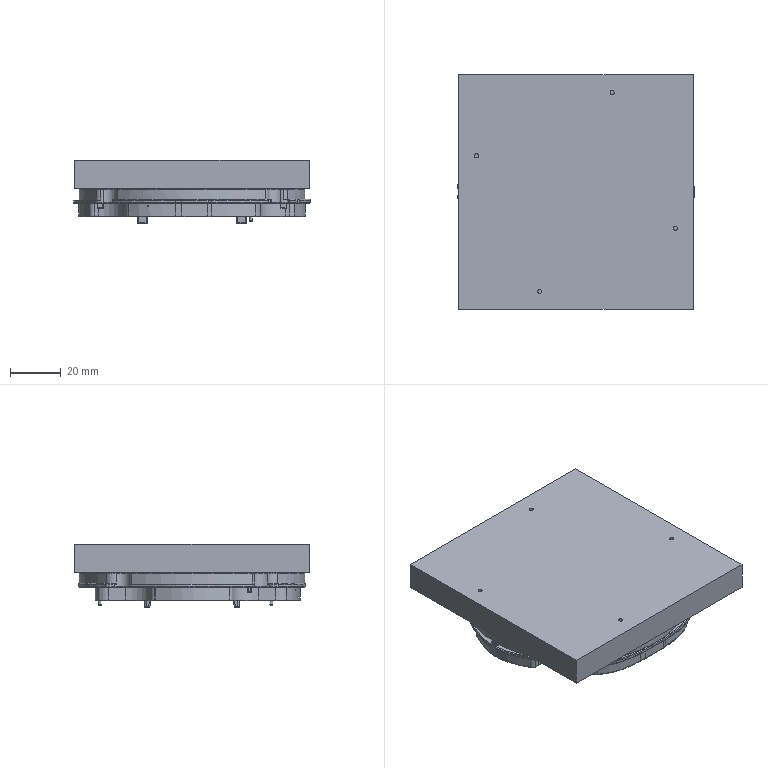NC program | NX | posted with a generic post | part box 92.935 x 92.1 x 24.829 mm
Lines 20379 to 21644 of 39008:
(PLANAR_MILL_5 , TOOL : D2-6-D4-50-3T-ROUGH)
N40738 T19 M6
N40740 G54
N40742 G17 G0 G90 X-18.001 Y31.511 S4500 M3
N40744 G43 Z20. H19
N40746 Z-3.15
N40748 G94 G1 Z-6.15 F1200.
N40750 X-16.001
N40752 X22.11
N40754 G2 X21.293 Y32.011 R2.814
N40756 G1 X-16.001
N40758 X-18.001
N40760 Z-3.15
N40762 G0 Z20.
N40764 Y27.511
N40766 Z-3.15
N40768 G1 Z-6.15
N40770 X-16.001
N40772 X24.224
N40774 Y28.011
N40776 X-16.001
N40778 X-18.001
N40780 Z-3.15
N40782 G0 Z20.
N40784 X-10.2 Y20.011
N40786 Z-3.15
N40788 G1 Z-6.15
N40790 X-12.2
N40792 X-22.92
N40794 G2 X-23.664 Y19.499 R3.
N40796 G1 X-12.2
N40798 X-10.2
N40800 Z-3.15
N40802 G0 Z20.
N40804 Y12.011
N40806 Z-3.15
N40808 G1 Z-6.15
N40810 X-12.2
N40812 X-38.698
N40814 G3 X-38.895 Y11.588 R81.553
N40816 G1 X-38.93 Y11.511
N40818 X-12.2
N40820 X-10.2
N40822 Z-3.15
N40824 G0 Z20.
N40826 Y8.011
N40828 Z-3.15
N40830 G1 Z-6.15
N40832 X-12.2
N40834 X-40.408
N40836 X-40.446 Y7.907
N40838 X-40.491 Y7.785
N40840 X-40.536 Y7.662
N40842 X-40.59 Y7.511
N40844 X-12.2
N40846 X-10.2
N40848 Z-3.15
N40850 G0 Z20.
N40852 Y4.011
N40854 Z-3.15
N40856 G1 Z-6.15
N40858 X-12.2
N40860 X-41.583
N40862 X-41.598 Y3.939
N40864 X-41.621 Y3.819
N40866 X-41.644 Y3.7
N40868 X-41.666 Y3.58
N40870 X-41.679 Y3.511
N40872 X-12.2
N40874 X-10.2
N40876 Z-3.15
N40878 G0 Z20.
N40880 Y0.011
N40882 Z-3.15
N40884 G1 Z-6.15
N40886 X-12.2
N40888 X-42.001 Y0.01
N40890 X-42. Y-0.108
N40892 X-41.999 Y-0.227
N40894 X-41.997 Y-0.345
N40896 X-41.994 Y-0.489
N40898 X-12.2
N40900 X-10.2
N40902 Z-3.15
N40904 G0 Z20.
N40906 Y-3.989
N40908 Z-3.15
N40910 G1 Z-6.15
N40912 X-12.2
N40914 X-41.59
N40916 X-41.58 Y-4.038
N40918 X-41.555 Y-4.157
N40920 X-41.53 Y-4.277
N40922 X-41.503 Y-4.397
N40924 X-41.483 Y-4.489
N40926 X-12.2
N40928 X-10.2
N40930 Z-3.15
N40932 G0 Z20.
N40934 Y-7.989
N40936 Z-3.15
N40938 G1 Z-6.15
N40940 X-12.2
N40942 X-40.418
N40944 G3 X-40.227 Y-8.489 R42.167
N40946 G1 X-12.2
N40948 X-10.2
N40950 Z-3.15
N40952 G0 Z20.
N40954 Y-11.989
N40956 Z-3.15
N40958 G1 Z-6.15
N40960 X-12.2
N40962 X-38.71
N40964 G3 X-38.474 Y-12.489 R107.874
N40966 G1 X-12.2
N40968 X-10.2
N40970 Z-3.15
N40972 G0 Z20.
N40974 X15.3
N40976 Z-3.15
N40978 G1 Z-6.15
N40980 X17.3
N40982 X38.475
N40984 G3 X38.711 Y-11.989 R103.852
N40986 G1 X17.3
N40988 X15.3
N40990 Z-3.15
N40992 G0 Z20.
N40994 Y-8.489
N40996 Z-3.15
N40998 G1 Z-6.15
N41000 X17.3
N41002 X40.228
N41004 G3 X40.419 Y-7.989 R42.476
N41006 G1 X17.3
N41008 X15.3
N41010 Z-3.15
N41012 G0 Z20.
N41014 Y-4.489
N41016 Z-3.15
N41018 G1 Z-6.15
N41020 X17.3
N41022 X41.483
N41024 X41.504 Y-4.397
N41026 X41.53 Y-4.278
N41028 X41.556 Y-4.158
N41030 X41.581 Y-4.038
N41032 X41.591 Y-3.989
N41034 X17.3
N41036 X15.3
N41038 Z-3.15
N41040 G0 Z20.
N41042 Y-0.489
N41044 Z-3.15
N41046 G1 Z-6.15
N41048 X17.3
N41050 X41.997
N41052 X41.998 Y-0.464
N41054 X42. Y-0.345
N41056 X42.002 Y-0.226
N41058 X42.003 Y-0.108
N41060 Y0.011
N41062 X17.3
N41064 X15.3
N41066 Z-3.15
N41068 G0 Z20.
N41070 Y3.511
N41072 Z-3.15
N41074 G1 Z-6.15
N41076 X17.3
N41078 X41.684
N41080 X41.671 Y3.58
N41082 X41.649 Y3.699
N41084 X41.626 Y3.819
N41086 X41.603 Y3.939
N41088 X41.588 Y4.011
N41090 X17.3
N41092 X15.3
N41094 Z-3.15
N41096 G0 Z20.
N41098 Y7.511
N41100 Z-3.15
N41102 G1 Z-6.15
N41104 X17.3
N41106 X40.595
N41108 X40.584 Y7.542
N41110 X40.54 Y7.664
N41112 X40.496 Y7.786
N41114 X40.451 Y7.907
N41116 X40.412 Y8.011
N41118 X17.3
N41120 X15.3
N41122 Z-3.15
N41124 G0 Z20.
N41126 Y11.511
N41128 Z-3.15
N41130 G1 Z-6.15
N41132 X17.3
N41134 X38.935
N41136 G3 X38.841 Y11.713 R71.035
N41138 X38.702 Y12.011 R96.799
N41140 G1 X17.3
N41142 X15.3
N41144 Z-3.15
N41146 G0 Z20.
N41148 Y19.499
N41150 Z-3.15
N41152 G1 Z-6.15
N41154 X18.001
N41156 X26.017
N41158 G2 X25.725 Y20.011 R12.5
N41160 G1 X17.3
N41162 X15.3
N41164 Z-3.15
N41166 G0 Z20.
N41168 Y19.499
N41170 Z-3.275
N41172 G1 Z-6.275
N41174 X18.001
N41176 X26.017
N41178 G2 X25.725 Y20.011 R12.5
N41180 G1 X17.3
N41182 X15.3
N41184 Z-3.275
N41186 G0 Z20.
N41188 Y11.511
N41190 Z-3.275
N41192 G1 Z-6.275
N41194 X17.3
N41196 X38.935
N41198 G3 X38.841 Y11.713 R71.035
N41200 X38.702 Y12.011 R96.799
N41202 G1 X17.3
N41204 X15.3
N41206 Z-3.275
N41208 G0 Z20.
N41210 Y7.511
N41212 Z-3.275
N41214 G1 Z-6.275
N41216 X17.3
N41218 X40.595
N41220 X40.584 Y7.542
N41222 X40.54 Y7.664
N41224 X40.496 Y7.786
N41226 X40.451 Y7.907
N41228 X40.412 Y8.011
N41230 X17.3
N41232 X15.3
N41234 Z-3.275
N41236 G0 Z20.
N41238 Y3.511
N41240 Z-3.275
N41242 G1 Z-6.275
N41244 X17.3
N41246 X41.684
N41248 X41.671 Y3.58
N41250 X41.649 Y3.699
N41252 X41.626 Y3.819
N41254 X41.603 Y3.939
N41256 X41.588 Y4.011
N41258 X17.3
N41260 X15.3
N41262 Z-3.275
N41264 G0 Z20.
N41266 Y-0.489
N41268 Z-3.275
N41270 G1 Z-6.275
N41272 X17.3
N41274 X41.997
N41276 X41.998 Y-0.464
N41278 X42. Y-0.345
N41280 X42.002 Y-0.226
N41282 X42.003 Y-0.108
N41284 Y0.011
N41286 X17.3
N41288 X15.3
N41290 Z-3.275
N41292 G0 Z20.
N41294 Y-4.489
N41296 Z-3.275
N41298 G1 Z-6.275
N41300 X17.3
N41302 X41.483
N41304 X41.504 Y-4.397
N41306 X41.53 Y-4.278
N41308 X41.556 Y-4.158
N41310 X41.581 Y-4.038
N41312 X41.591 Y-3.989
N41314 X17.3
N41316 X15.3
N41318 Z-3.275
N41320 G0 Z20.
N41322 Y-8.489
N41324 Z-3.275
N41326 G1 Z-6.275
N41328 X17.3
N41330 X40.228
N41332 G3 X40.419 Y-7.989 R42.476
N41334 G1 X17.3
N41336 X15.3
N41338 Z-3.275
N41340 G0 Z20.
N41342 Y-12.489
N41344 Z-3.275
N41346 G1 Z-6.275
N41348 X17.3
N41350 X38.475
N41352 G3 X38.711 Y-11.989 R103.852
N41354 G1 X17.3
N41356 X15.3
N41358 Z-3.275
N41360 G0 Z20.
N41362 X-10.2
N41364 Z-3.275
N41366 G1 Z-6.275
N41368 X-12.2
N41370 X-38.71
N41372 G3 X-38.474 Y-12.489 R107.874
N41374 G1 X-12.2
N41376 X-10.2
N41378 Z-3.275
N41380 G0 Z20.
N41382 Y-7.989
N41384 Z-3.275
N41386 G1 Z-6.275
N41388 X-12.2
N41390 X-40.418
N41392 G3 X-40.227 Y-8.489 R42.167
N41394 G1 X-12.2
N41396 X-10.2
N41398 Z-3.275
N41400 G0 Z20.
N41402 Y-3.989
N41404 Z-3.275
N41406 G1 Z-6.275
N41408 X-12.2
N41410 X-41.59
N41412 X-41.58 Y-4.038
N41414 X-41.555 Y-4.157
N41416 X-41.53 Y-4.277
N41418 X-41.503 Y-4.397
N41420 X-41.483 Y-4.489
N41422 X-12.2
N41424 X-10.2
N41426 Z-3.275
N41428 G0 Z20.
N41430 Y0.011
N41432 Z-3.275
N41434 G1 Z-6.275
N41436 X-12.2
N41438 X-42.001 Y0.01
N41440 X-42. Y-0.108
N41442 X-41.999 Y-0.227
N41444 X-41.997 Y-0.345
N41446 X-41.994 Y-0.489
N41448 X-12.2
N41450 X-10.2
N41452 Z-3.275
N41454 G0 Z20.
N41456 Y4.011
N41458 Z-3.275
N41460 G1 Z-6.275
N41462 X-12.2
N41464 X-41.583
N41466 X-41.598 Y3.939
N41468 X-41.621 Y3.819
N41470 X-41.644 Y3.7
N41472 X-41.666 Y3.58
N41474 X-41.679 Y3.511
N41476 X-12.2
N41478 X-10.2
N41480 Z-3.275
N41482 G0 Z20.
N41484 Y8.011
N41486 Z-3.275
N41488 G1 Z-6.275
N41490 X-12.2
N41492 X-40.408
N41494 X-40.446 Y7.907
N41496 X-40.491 Y7.785
N41498 X-40.536 Y7.662
N41500 X-40.59 Y7.511
N41502 X-12.2
N41504 X-10.2
N41506 Z-3.275
N41508 G0 Z20.
N41510 Y12.011
N41512 Z-3.275
N41514 G1 Z-6.275
N41516 X-12.2
N41518 X-38.698
N41520 G3 X-38.895 Y11.588 R81.553
N41522 G1 X-38.93 Y11.511
N41524 X-12.2
N41526 X-10.2
N41528 Z-3.275
N41530 G0 Z20.
N41532 Y20.011
N41534 Z-3.275
N41536 G1 Z-6.275
N41538 X-12.2
N41540 X-22.92
N41542 G2 X-23.664 Y19.499 R3.
N41544 G1 X-12.2
N41546 X-10.2
N41548 Z-3.275
N41550 G0 Z20.
N41552 X-18.001 Y27.511
N41554 Z-3.275
N41556 G1 Z-6.275
N41558 X-16.001
N41560 X24.224
N41562 Y28.011
N41564 X-16.001
N41566 X-18.001
N41568 Z-3.275
N41570 G0 Z20.
N41572 Y31.511
N41574 Z-3.275
N41576 G1 Z-6.275
N41578 X-16.001
N41580 X22.11
N41582 G2 X21.293 Y32.011 R2.814
N41584 G1 X-16.001
N41586 X-18.001
N41588 Z-3.275
N41590 G0 Z20.
N41592 Y31.511
N41594 Z-3.4
N41596 G1 Z-6.4
N41598 X-16.001
N41600 X22.11
N41602 G2 X21.293 Y32.011 R2.814
N41604 G1 X-16.001
N41606 X-18.001
N41608 Z-3.4
N41610 G0 Z20.
N41612 Y27.511
N41614 Z-3.4
N41616 G1 Z-6.4
N41618 X-16.001
N41620 X24.224
N41622 Y28.011
N41624 X-16.001
N41626 X-18.001
N41628 Z-3.4
N41630 G0 Z20.
N41632 X-10.2 Y20.011
N41634 Z-3.4
N41636 G1 Z-6.4
N41638 X-12.2
N41640 X-22.92
N41642 G2 X-23.664 Y19.499 R3.
N41644 G1 X-12.2
N41646 X-10.2
N41648 Z-3.4
N41650 G0 Z20.
N41652 Y12.011
N41654 Z-3.4
N41656 G1 Z-6.4
N41658 X-12.2
N41660 X-38.698
N41662 G3 X-38.895 Y11.588 R81.553
N41664 G1 X-38.93 Y11.511
N41666 X-12.2
N41668 X-10.2
N41670 Z-3.4
N41672 G0 Z20.
N41674 Y8.011
N41676 Z-3.4
N41678 G1 Z-6.4
N41680 X-12.2
N41682 X-40.408
N41684 X-40.446 Y7.907
N41686 X-40.491 Y7.785
N41688 X-40.536 Y7.662
N41690 X-40.59 Y7.511
N41692 X-12.2
N41694 X-10.2
N41696 Z-3.4
N41698 G0 Z20.
N41700 Y4.011
N41702 Z-3.4
N41704 G1 Z-6.4
N41706 X-12.2
N41708 X-41.583
N41710 X-41.598 Y3.939
N41712 X-41.621 Y3.819
N41714 X-41.644 Y3.7
N41716 X-41.666 Y3.58
N41718 X-41.679 Y3.511
N41720 X-12.2
N41722 X-10.2
N41724 Z-3.4
N41726 G0 Z20.
N41728 Y0.011
N41730 Z-3.4
N41732 G1 Z-6.4
N41734 X-12.2
N41736 X-42.001 Y0.01
N41738 X-42. Y-0.108
N41740 X-41.999 Y-0.227
N41742 X-41.997 Y-0.345
N41744 X-41.994 Y-0.489
N41746 X-12.2
N41748 X-10.2
N41750 Z-3.4
N41752 G0 Z20.
N41754 Y-3.989
N41756 Z-3.4
N41758 G1 Z-6.4
N41760 X-12.2
N41762 X-41.59
N41764 X-41.58 Y-4.038
N41766 X-41.555 Y-4.157
N41768 X-41.53 Y-4.277
N41770 X-41.503 Y-4.397
N41772 X-41.483 Y-4.489
N41774 X-12.2
N41776 X-10.2
N41778 Z-3.4
N41780 G0 Z20.
N41782 Y-7.989
N41784 Z-3.4
N41786 G1 Z-6.4
N41788 X-12.2
N41790 X-40.418
N41792 G3 X-40.227 Y-8.489 R42.167
N41794 G1 X-12.2
N41796 X-10.2
N41798 Z-3.4
N41800 G0 Z20.
N41802 Y-11.989
N41804 Z-3.4
N41806 G1 Z-6.4
N41808 X-12.2
N41810 X-38.71
N41812 G3 X-38.474 Y-12.489 R107.874
N41814 G1 X-12.2
N41816 X-10.2
N41818 Z-3.4
N41820 G0 Z20.
N41822 X15.3
N41824 Z-3.4
N41826 G1 Z-6.4
N41828 X17.3
N41830 X38.475
N41832 G3 X38.711 Y-11.989 R103.852
N41834 G1 X17.3
N41836 X15.3
N41838 Z-3.4
N41840 G0 Z20.
N41842 Y-8.489
N41844 Z-3.4
N41846 G1 Z-6.4
N41848 X17.3
N41850 X40.228
N41852 G3 X40.419 Y-7.989 R42.476
N41854 G1 X17.3
N41856 X15.3
N41858 Z-3.4
N41860 G0 Z20.
N41862 Y-4.489
N41864 Z-3.4
N41866 G1 Z-6.4
N41868 X17.3
N41870 X41.483
N41872 X41.504 Y-4.397
N41874 X41.53 Y-4.278
N41876 X41.556 Y-4.158
N41878 X41.581 Y-4.038
N41880 X41.591 Y-3.989
N41882 X17.3
N41884 X15.3
N41886 Z-3.4
N41888 G0 Z20.
N41890 Y-0.489
N41892 Z-3.4
N41894 G1 Z-6.4
N41896 X17.3
N41898 X41.997
N41900 X41.998 Y-0.464
N41902 X42. Y-0.345
N41904 X42.002 Y-0.226
N41906 X42.003 Y-0.108
N41908 Y0.011
N41910 X17.3
N41912 X15.3
N41914 Z-3.4
N41916 G0 Z20.
N41918 Y3.511
N41920 Z-3.4
N41922 G1 Z-6.4
N41924 X17.3
N41926 X41.684
N41928 X41.671 Y3.58
N41930 X41.649 Y3.699
N41932 X41.626 Y3.819
N41934 X41.603 Y3.939
N41936 X41.588 Y4.011
N41938 X17.3
N41940 X15.3
N41942 Z-3.4
N41944 G0 Z20.
N41946 Y7.511
N41948 Z-3.4
N41950 G1 Z-6.4
N41952 X17.3
N41954 X40.595
N41956 X40.584 Y7.542
N41958 X40.54 Y7.664
N41960 X40.496 Y7.786
N41962 X40.451 Y7.907
N41964 X40.412 Y8.011
N41966 X17.3
N41968 X15.3
N41970 Z-3.4
N41972 G0 Z20.
N41974 Y11.511
N41976 Z-3.4
N41978 G1 Z-6.4
N41980 X17.3
N41982 X38.935
N41984 G3 X38.841 Y11.713 R71.035
N41986 X38.702 Y12.011 R96.799
N41988 G1 X17.3
N41990 X15.3
N41992 Z-3.4
N41994 G0 Z20.
N41996 Y19.499
N41998 Z-3.4
N42000 G1 Z-6.4
N42002 X18.001
N42004 X26.017
N42006 G2 X25.725 Y20.011 R12.5
N42008 G1 X17.3
N42010 X15.3
N42012 Z-3.4
N42014 G0 Z20.
N42016 Y19.499
N42018 Z-3.525
N42020 G1 Z-6.525
N42022 X18.001
N42024 X26.017
N42026 G2 X25.725 Y20.011 R12.5
N42028 G1 X17.3
N42030 X15.3
N42032 Z-3.525
N42034 G0 Z20.
N42036 Y11.511
N42038 Z-3.525
N42040 G1 Z-6.525
N42042 X17.3
N42044 X38.935
N42046 G3 X38.841 Y11.713 R71.035
N42048 X38.702 Y12.011 R96.799
N42050 G1 X17.3
N42052 X15.3
N42054 Z-3.525
N42056 G0 Z20.
N42058 Y7.511
N42060 Z-3.525
N42062 G1 Z-6.525
N42064 X17.3
N42066 X40.595
N42068 X40.584 Y7.542
N42070 X40.54 Y7.664
N42072 X40.496 Y7.786
N42074 X40.451 Y7.907
N42076 X40.412 Y8.011
N42078 X17.3
N42080 X15.3
N42082 Z-3.525
N42084 G0 Z20.
N42086 Y3.511
N42088 Z-3.525
N42090 G1 Z-6.525
N42092 X17.3
N42094 X41.684
N42096 X41.671 Y3.58
N42098 X41.649 Y3.699
N42100 X41.626 Y3.819
N42102 X41.603 Y3.939
N42104 X41.588 Y4.011
N42106 X17.3
N42108 X15.3
N42110 Z-3.525
N42112 G0 Z20.
N42114 Y-0.489
N42116 Z-3.525
N42118 G1 Z-6.525
N42120 X17.3
N42122 X41.997
N42124 X41.998 Y-0.464
N42126 X42. Y-0.345
N42128 X42.002 Y-0.226
N42130 X42.003 Y-0.108
N42132 Y0.011
N42134 X17.3
N42136 X15.3
N42138 Z-3.525
N42140 G0 Z20.
N42142 Y-4.489
N42144 Z-3.525
N42146 G1 Z-6.525
N42148 X17.3
N42150 X41.483
N42152 X41.504 Y-4.397
N42154 X41.53 Y-4.278
N42156 X41.556 Y-4.158
N42158 X41.581 Y-4.038
N42160 X41.591 Y-3.989
N42162 X17.3
N42164 X15.3
N42166 Z-3.525
N42168 G0 Z20.
N42170 Y-8.489
N42172 Z-3.525
N42174 G1 Z-6.525
N42176 X17.3
N42178 X40.228
N42180 G3 X40.419 Y-7.989 R42.476
N42182 G1 X17.3
N42184 X15.3
N42186 Z-3.525
N42188 G0 Z20.
N42190 Y-12.489
N42192 Z-3.525
N42194 G1 Z-6.525
N42196 X17.3
N42198 X38.475
N42200 G3 X38.711 Y-11.989 R103.852
N42202 G1 X17.3
N42204 X15.3
N42206 Z-3.525
N42208 G0 Z20.
N42210 X-10.2
N42212 Z-3.525
N42214 G1 Z-6.525
N42216 X-12.2
N42218 X-38.71
N42220 G3 X-38.474 Y-12.489 R107.874
N42222 G1 X-12.2
N42224 X-10.2
N42226 Z-3.525
N42228 G0 Z20.
N42230 Y-7.989
N42232 Z-3.525
N42234 G1 Z-6.525
N42236 X-12.2
N42238 X-40.418
N42240 G3 X-40.227 Y-8.489 R42.167
N42242 G1 X-12.2
N42244 X-10.2
N42246 Z-3.525
N42248 G0 Z20.
N42250 Y-3.989
N42252 Z-3.525
N42254 G1 Z-6.525
N42256 X-12.2
N42258 X-41.59
N42260 X-41.58 Y-4.038
N42262 X-41.555 Y-4.157
N42264 X-41.53 Y-4.277
N42266 X-41.503 Y-4.397
N42268 X-41.483 Y-4.489
N42270 X-12.2
N42272 X-10.2
N42274 Z-3.525
N42276 G0 Z20.
N42278 Y0.011
N42280 Z-3.525
N42282 G1 Z-6.525
N42284 X-12.2
N42286 X-42.001 Y0.01
N42288 X-42. Y-0.108
N42290 X-41.999 Y-0.227
N42292 X-41.997 Y-0.345
N42294 X-41.994 Y-0.489
N42296 X-12.2
N42298 X-10.2
N42300 Z-3.525
N42302 G0 Z20.
N42304 Y4.011
N42306 Z-3.525
N42308 G1 Z-6.525
N42310 X-12.2
N42312 X-41.583
N42314 X-41.598 Y3.939
N42316 X-41.621 Y3.819
N42318 X-41.644 Y3.7
N42320 X-41.666 Y3.58
N42322 X-41.679 Y3.511
N42324 X-12.2
N42326 X-10.2
N42328 Z-3.525
N42330 G0 Z20.
N42332 Y8.011
N42334 Z-3.525
N42336 G1 Z-6.525
N42338 X-12.2
N42340 X-40.408
N42342 X-40.446 Y7.907
N42344 X-40.491 Y7.785
N42346 X-40.536 Y7.662
N42348 X-40.59 Y7.511
N42350 X-12.2
N42352 X-10.2
N42354 Z-3.525
N42356 G0 Z20.
N42358 Y12.011
N42360 Z-3.525
N42362 G1 Z-6.525
N42364 X-12.2
N42366 X-38.698
N42368 G3 X-38.895 Y11.588 R81.553
N42370 G1 X-38.93 Y11.511
N42372 X-12.2
N42374 X-10.2
N42376 Z-3.525
N42378 G0 Z20.
N42380 Y20.011
N42382 Z-3.525
N42384 G1 Z-6.525
N42386 X-12.2
N42388 X-22.92
N42390 G2 X-23.664 Y19.499 R3.
N42392 G1 X-12.2
N42394 X-10.2
N42396 Z-3.525
N42398 G0 Z20.
N42400 X-18.001 Y27.511
N42402 Z-3.525
N42404 G1 Z-6.525
N42406 X-16.001
N42408 X24.224
N42410 Y28.011
N42412 X-16.001
N42414 X-18.001
N42416 Z-3.525
N42418 G0 Z20.
N42420 Y31.511
N42422 Z-3.525
N42424 G1 Z-6.525
N42426 X-16.001
N42428 X22.11
N42430 G2 X21.293 Y32.011 R2.814
N42432 G1 X-16.001
N42434 X-18.001
N42436 Z-3.525
N42438 G0 Z20.
(PLANAR_MILL_6 , TOOL : D2-6-D4-50-3T-ROUGH)
N42440 X-11.763 Y23.511
N42442 Z-5.025
N42444 G1 X1.096 Z-6.15
N42446 X24.465
N42448 G2 X24.376 Y24.011 R12.5
N42450 G1 X-17.293
N42452 G2 X-17.501 Y24.002 R2.5
N42454 G1 X-22.573
N42456 G2 X-22.273 Y23.511 R3.
N42458 G1 X1.096
N42460 Z-5.15
N42462 G0 Z20.
N42464 X-11.763
N42466 Z-5.15
N42468 G1 X1.096 Z-6.275
N42470 X24.465
N42472 G2 X24.376 Y24.011 R12.5
N42474 G1 X-17.293
N42476 G2 X-17.501 Y24.002 R2.5
N42478 G1 X-22.573
N42480 G2 X-22.273 Y23.511 R3.
N42482 G1 X1.096
N42484 Z-5.275
N42486 G0 Z20.
N42488 X-11.763
N42490 Z-5.275
N42492 G1 X1.096 Z-6.4
N42494 X24.465
N42496 G2 X24.376 Y24.011 R12.5
N42498 G1 X-17.293
N42500 G2 X-17.501 Y24.002 R2.5
N42502 G1 X-22.573
N42504 G2 X-22.273 Y23.511 R3.
N42506 G1 X1.096
N42508 Z-5.4
N42510 G0 Z20.
N42512 X-11.763
N42514 Z-5.4
N42516 G1 X1.096 Z-6.525
N42518 X24.465
N42520 G2 X24.376 Y24.011 R12.5
N42522 G1 X-17.293
N42524 G2 X-17.501 Y24.002 R2.5
N42526 G1 X-22.573
N42528 G2 X-22.273 Y23.511 R3.
N42530 G1 X1.096
N42532 Z-5.525
N42534 G0 Z20.
(PLANAR_MILL_6_COPY , TOOL : D2-6-D4-50-3T-ROUGH)
N42536 X13.064 Y-35.989
N42538 Z-5.025
N42540 G1 X0.001 Z-6.168
N42542 X-20.804
N42544 G3 X-20.656 Y-36.489 R1.
N42546 G1 X20.657
N42548 G3 X20.806 Y-35.989 R1.
N42550 G1 X0.001
N42552 Z-5.168
N42554 G0 Z20.
N42556 X13.064
N42558 Z-5.168
N42560 G1 X0.001 Z-6.311
N42562 X-20.804
N42564 G3 X-20.656 Y-36.489 R1.
N42566 G1 X20.657
N42568 G3 X20.806 Y-35.989 R1.
N42570 G1 X0.001
N42572 Z-5.311
N42574 G0 Z20.
N42576 X13.064
N42578 Z-5.311
N42580 G1 X0.001 Z-6.454
N42582 X-20.804
N42584 G3 X-20.656 Y-36.489 R1.
N42586 G1 X20.657
N42588 G3 X20.806 Y-35.989 R1.
N42590 G1 X0.001
N42592 Z-5.454
N42594 G0 Z20.
N42596 X13.064
N42598 Z-5.454
N42600 G1 X0.001 Z-6.597
N42602 X-20.804
N42604 G3 X-20.656 Y-36.489 R1.
N42606 G1 X20.657
N42608 G3 X20.806 Y-35.989 R1.
N42610 G1 X0.001
N42612 Z-5.597
N42614 G0 Z20.
N42616 X13.064
N42618 Z-5.597
N42620 G1 X0.001 Z-6.74
N42622 X-20.804
N42624 G3 X-20.656 Y-36.489 R1.
N42626 G1 X20.657
N42628 G3 X20.806 Y-35.989 R1.
N42630 G1 X0.001
N42632 Z-5.74
N42634 G0 Z20.
N42636 X13.064
N42638 Z-5.74
N42640 G1 X0.001 Z-6.883
N42642 X-20.804
N42644 G3 X-20.656 Y-36.489 R1.
N42646 G1 X20.657
N42648 G3 X20.806 Y-35.989 R1.
N42650 G1 X0.001
N42652 Z-5.883
N42654 G0 Z20.
N42656 X13.064
N42658 Z-5.883
N42660 G1 X0.001 Z-7.025
N42662 X-20.804
N42664 G3 X-20.656 Y-36.489 R1.
N42666 G1 X20.657
N42668 G3 X20.806 Y-35.989 R1.
N42670 G1 X0.001
N42672 Z-6.025
N42674 G0 Z20.
N42676 X13.139 Y-31.989
N42678 Z-5.025
N42680 G1 X0.076 Z-6.168
N42682 X-21.167
N42684 G3 X-21.045 Y-32.256 R0.5
N42686 G2 X-20.858 Y-32.489 R2.814
N42688 G1 X20.861
N42690 G2 X21.319 Y-31.989 R2.814
N42692 G1 X0.076
N42694 Z-5.168
N42696 G0 Z20.
N42698 X13.139
N42700 Z-5.168
N42702 G1 X0.076 Z-6.311
N42704 X-21.167
N42706 G3 X-21.045 Y-32.256 R0.5
N42708 G2 X-20.858 Y-32.489 R2.814
N42710 G1 X20.861
N42712 G2 X21.319 Y-31.989 R2.814
N42714 G1 X0.076
N42716 Z-5.311
N42718 G0 Z20.
N42720 X13.139
N42722 Z-5.311
N42724 G1 X0.076 Z-6.454
N42726 X-21.167
N42728 G3 X-21.045 Y-32.256 R0.5
N42730 G2 X-20.858 Y-32.489 R2.814
N42732 G1 X20.861
N42734 G2 X21.319 Y-31.989 R2.814
N42736 G1 X0.076
N42738 Z-5.454
N42740 G0 Z20.
N42742 X13.139
N42744 Z-5.454
N42746 G1 X0.076 Z-6.597
N42748 X-21.167
N42750 G3 X-21.045 Y-32.256 R0.5
N42752 G2 X-20.858 Y-32.489 R2.814
N42754 G1 X20.861
N42756 G2 X21.319 Y-31.989 R2.814
N42758 G1 X0.076
N42760 Z-5.597
N42762 G0 Z20.
N42764 X13.139
N42766 Z-5.597
N42768 G1 X0.076 Z-6.74
N42770 X-21.167
N42772 G3 X-21.045 Y-32.256 R0.5
N42774 G2 X-20.858 Y-32.489 R2.814
N42776 G1 X20.861
N42778 G2 X21.319 Y-31.989 R2.814
N42780 G1 X0.076
N42782 Z-5.74
N42784 G0 Z20.
N42786 X13.139
N42788 Z-5.74
N42790 G1 X0.076 Z-6.883
N42792 X-21.167
N42794 G3 X-21.045 Y-32.256 R0.5
N42796 G2 X-20.858 Y-32.489 R2.814
N42798 G1 X20.861
N42800 G2 X21.319 Y-31.989 R2.814
N42802 G1 X0.076
N42804 Z-5.883
N42806 G0 Z20.
N42808 X13.139
N42810 Z-5.883
N42812 G1 X0.076 Z-7.025
N42814 X-21.167
N42816 G3 X-21.045 Y-32.256 R0.5
N42818 G2 X-20.858 Y-32.489 R2.814
N42820 G1 X20.861
N42822 G2 X21.319 Y-31.989 R2.814
N42824 G1 X0.076
N42826 Z-6.025
N42828 G0 Z20.
N42830 X13.064 Y-27.989
N42832 Z-5.025
N42834 G1 X0.001 Z-6.168
N42836 X-24.221
N42838 Y-28.489
N42840 X24.224
N42842 Y-27.989
N42844 X0.001
N42846 Z-5.168
N42848 G0 Z20.
N42850 X13.064
N42852 Z-5.168
N42854 G1 X0.001 Z-6.311
N42856 X-24.221
N42858 Y-28.489
N42860 X24.224
N42862 Y-27.989
N42864 X0.001
N42866 Z-5.311
N42868 G0 Z20.
N42870 X13.064
N42872 Z-5.311
N42874 G1 X0.001 Z-6.454
N42876 X-24.221
N42878 Y-28.489
N42880 X24.224
N42882 Y-27.989
N42884 X0.001
N42886 Z-5.454
N42888 G0 Z20.
N42890 X13.064
N42892 Z-5.454
N42894 G1 X0.001 Z-6.597
N42896 X-24.221
N42898 Y-28.489
N42900 X24.224
N42902 Y-27.989
N42904 X0.001
N42906 Z-5.597
N42908 G0 Z20.
N42910 X13.064
N42912 Z-5.597
N42914 G1 X0.001 Z-6.74
N42916 X-24.221
N42918 Y-28.489
N42920 X24.224
N42922 Y-27.989
N42924 X0.001
N42926 Z-5.74
N42928 G0 Z20.
N42930 X13.064
N42932 Z-5.74
N42934 G1 X0.001 Z-6.883
N42936 X-24.221
N42938 Y-28.489
N42940 X24.224
N42942 Y-27.989
N42944 X0.001
N42946 Z-5.883
N42948 G0 Z20.
N42950 X13.064
N42952 Z-5.883
N42954 G1 X0.001 Z-7.025
N42956 X-24.221
N42958 Y-28.489
N42960 X24.224
N42962 Y-27.989
N42964 X0.001
N42966 Z-6.025
N42968 G0 Z20.
N42970 X13.064 Y-23.989
N42972 Z-5.025
N42974 G1 X0.001 Z-6.168
N42976 X-24.376
N42978 G2 X-24.307 Y-24.489 R12.5
N42980 G1 X24.31
N42982 G2 X24.379 Y-23.989 R12.5
N42984 G1 X0.001
N42986 Z-5.168
N42988 G0 Z20.
N42990 X13.064
N42992 Z-5.168
N42994 G1 X0.001 Z-6.311
N42996 X-24.376
N42998 G2 X-24.307 Y-24.489 R12.5
N43000 G1 X24.31
N43002 G2 X24.379 Y-23.989 R12.5
N43004 G1 X0.001
N43006 Z-5.311
N43008 G0 Z20.
N43010 X13.064
N43012 Z-5.311
N43014 G1 X0.001 Z-6.454
N43016 X-24.376
N43018 G2 X-24.307 Y-24.489 R12.5
N43020 G1 X24.31
N43022 G2 X24.379 Y-23.989 R12.5
N43024 G1 X0.001
N43026 Z-5.454
N43028 G0 Z20.
N43030 X13.064
N43032 Z-5.454
N43034 G1 X0.001 Z-6.597
N43036 X-24.376
N43038 G2 X-24.307 Y-24.489 R12.5
N43040 G1 X24.31
N43042 G2 X24.379 Y-23.989 R12.5
N43044 G1 X0.001
N43046 Z-5.597
N43048 G0 Z20.
N43050 X13.064
N43052 Z-5.597
N43054 G1 X0.001 Z-6.74
N43056 X-24.376
N43058 G2 X-24.307 Y-24.489 R12.5
N43060 G1 X24.31
N43062 G2 X24.379 Y-23.989 R12.5
N43064 G1 X0.001
N43066 Z-5.74
N43068 G0 Z20.
N43070 X13.064
N43072 Z-5.74
N43074 G1 X0.001 Z-6.883
N43076 X-24.376
N43078 G2 X-24.307 Y-24.489 R12.5
N43080 G1 X24.31
N43082 G2 X24.379 Y-23.989 R12.5
N43084 G1 X0.001
N43086 Z-5.883
N43088 G0 Z20.
N43090 X13.064
N43092 Z-5.883
N43094 G1 X0.001 Z-7.025
N43096 X-24.376
N43098 G2 X-24.307 Y-24.489 R12.5
N43100 G1 X24.31
N43102 G2 X24.379 Y-23.989 R12.5
N43104 G1 X0.001
N43106 Z-6.025
N43108 G0 Z20.
N43110 X13.064 Y-19.989
N43112 Z-5.025
N43114 G1 X0.001 Z-6.168
N43116 X-25.735
N43118 G2 X-25.478 Y-20.489 R12.5
N43120 G1 X25.481
N43122 G2 X25.738 Y-19.989 R12.5
N43124 G1 X0.001
N43126 Z-5.168
N43128 G0 Z20.
N43130 X13.064
N43132 Z-5.168
N43134 G1 X0.001 Z-6.311
N43136 X-25.735
N43138 G2 X-25.478 Y-20.489 R12.5
N43140 G1 X25.481
N43142 G2 X25.738 Y-19.989 R12.5
N43144 G1 X0.001
N43146 Z-5.311
N43148 G0 Z20.
N43150 X13.064
N43152 Z-5.311
N43154 G1 X0.001 Z-6.454
N43156 X-25.735
N43158 G2 X-25.478 Y-20.489 R12.5
N43160 G1 X25.481
N43162 G2 X25.738 Y-19.989 R12.5
N43164 G1 X0.001
N43166 Z-5.454
N43168 G0 Z20.
N43170 X13.064
N43172 Z-5.454
N43174 G1 X0.001 Z-6.597
N43176 X-25.735
N43178 G2 X-25.478 Y-20.489 R12.5
N43180 G1 X25.481
N43182 G2 X25.738 Y-19.989 R12.5
N43184 G1 X0.001
N43186 Z-5.597
N43188 G0 Z20.
N43190 X13.064
N43192 Z-5.597
N43194 G1 X0.001 Z-6.74
N43196 X-25.735
N43198 G2 X-25.478 Y-20.489 R12.5
N43200 G1 X25.481
N43202 G2 X25.738 Y-19.989 R12.5
N43204 G1 X0.001
N43206 Z-5.74
N43208 G0 Z20.
N43210 X13.064
N43212 Z-5.74
N43214 G1 X0.001 Z-6.883
N43216 X-25.735
N43218 G2 X-25.478 Y-20.489 R12.5
N43220 G1 X25.481
N43222 G2 X25.738 Y-19.989 R12.5
N43224 G1 X0.001
N43226 Z-5.883
N43228 G0 Z20.
N43230 X13.064
N43232 Z-5.883
N43234 G1 X0.001 Z-7.025
N43236 X-25.735
N43238 G2 X-25.478 Y-20.489 R12.5
N43240 G1 X25.481
N43242 G2 X25.738 Y-19.989 R12.5
N43244 G1 X0.001
N43246 Z-6.025
N43248 G0 Z20.
N43250 M5